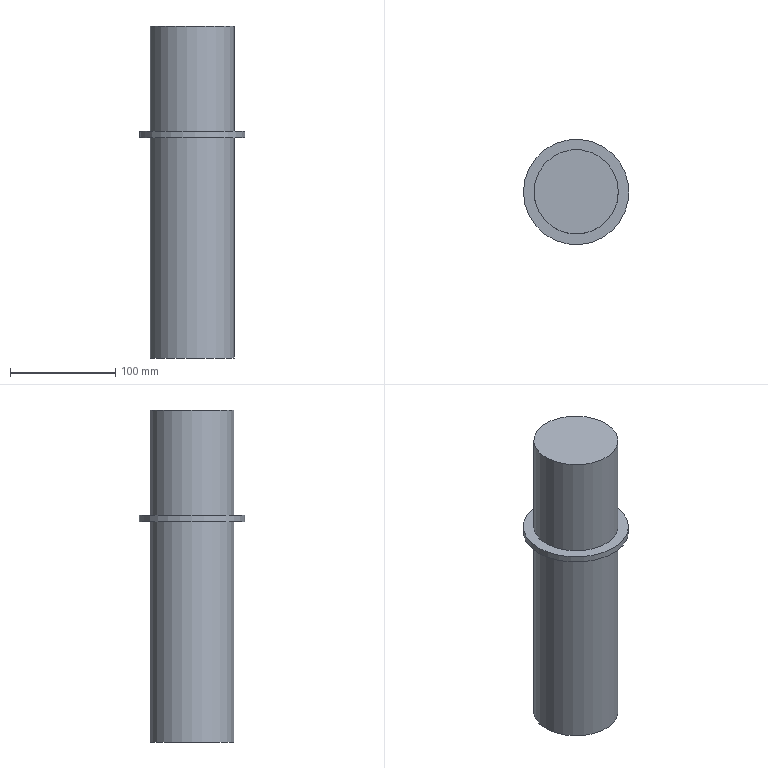Part | NX | features MAIN_BODY 2 | 1 solid | 7 faces | box 100 x 100 x 315 mm | volume 1600327 mm3 | plane 4 | cylinder 3 | commonest cylinder face diameters 80 x2 100 x1
STEP:
#1=CARTESIAN_POINT('',(-335.,-285.,370.));
#2=VERTEX_POINT('',#1);
#3=CARTESIAN_POINT('',(-295.,-285.,370.));
#4=DIRECTION('',(0.,0.,-1.));
#5=DIRECTION('',(-1.,0.,0.));
#6=AXIS2_PLACEMENT_3D('',#3,#4,#5);
#7=CIRCLE('',#6,40.);
#8=EDGE_CURVE('',#2,#2,#7,.T.);
#9=ORIENTED_EDGE('',*,*,#8,.F.);
#10=EDGE_LOOP('',(#9));
#11=FACE_BOUND('',#10,.T.);
#12=CARTESIAN_POINT('',(-255.,-285.,470.));
#13=VERTEX_POINT('',#12);
#14=CARTESIAN_POINT('',(-295.,-285.,470.));
#15=DIRECTION('',(0.,0.,1.));
#16=DIRECTION('',(1.,0.,0.));
#17=AXIS2_PLACEMENT_3D('',#14,#15,#16);
#18=CIRCLE('',#17,40.);
#19=EDGE_CURVE('',#13,#13,#18,.F.);
#20=ORIENTED_EDGE('',*,*,#19,.T.);
#21=EDGE_LOOP('',(#20));
#22=FACE_BOUND('',#21,.T.);
#23=CARTESIAN_POINT('',(-295.,-285.,463.));
#24=DIRECTION('',(0.,0.,-1.));
#25=DIRECTION('',(-1.,0.,0.));
#26=AXIS2_PLACEMENT_3D('',#23,#24,#25);
#27=CYLINDRICAL_SURFACE('',#26,40.);
#28=ADVANCED_FACE('',(#11,#22),#27,.T.);
#29=ORIENTED_EDGE('',*,*,#19,.F.);
#30=EDGE_LOOP('',(#29));
#31=FACE_BOUND('',#30,.T.);
#32=CARTESIAN_POINT('',(-295.,-285.,470.));
#33=DIRECTION('',(0.,0.,1.));
#34=DIRECTION('',(1.,0.,0.));
#35=AXIS2_PLACEMENT_3D('',#32,#33,#34);
#36=PLANE('',#35);
#37=ADVANCED_FACE('',(#31),#36,.T.);
#38=CARTESIAN_POINT('',(-345.,-285.,364.));
#39=VERTEX_POINT('',#38);
#40=CARTESIAN_POINT('',(-295.,-285.,364.));
#41=DIRECTION('',(0.,0.,-1.));
#42=DIRECTION('',(-1.,0.,0.));
#43=AXIS2_PLACEMENT_3D('',#40,#41,#42);
#44=CIRCLE('',#43,50.);
#45=EDGE_CURVE('',#39,#39,#44,.F.);
#46=ORIENTED_EDGE('',*,*,#45,.T.);
#47=EDGE_LOOP('',(#46));
#48=FACE_BOUND('',#47,.T.);
#49=CARTESIAN_POINT('',(-345.,-285.,370.));
#50=VERTEX_POINT('',#49);
#51=CARTESIAN_POINT('',(-295.,-285.,370.));
#52=DIRECTION('',(0.,0.,-1.));
#53=DIRECTION('',(-1.,0.,0.));
#54=AXIS2_PLACEMENT_3D('',#51,#52,#53);
#55=CIRCLE('',#54,50.);
#56=EDGE_CURVE('',#50,#50,#55,.F.);
#57=ORIENTED_EDGE('',*,*,#56,.F.);
#58=EDGE_LOOP('',(#57));
#59=FACE_BOUND('',#58,.T.);
#60=CARTESIAN_POINT('',(-295.,-285.,364.));
#61=DIRECTION('',(0.,0.,1.));
#62=DIRECTION('',(1.,0.,0.));
#63=AXIS2_PLACEMENT_3D('',#60,#61,#62);
#64=CYLINDRICAL_SURFACE('',#63,50.);
#65=ADVANCED_FACE('',(#48,#59),#64,.T.);
#66=CARTESIAN_POINT('',(-335.,-285.,364.));
#67=VERTEX_POINT('',#66);
#68=CARTESIAN_POINT('',(-295.,-285.,364.));
#69=DIRECTION('',(0.,0.,-1.));
#70=DIRECTION('',(-1.,0.,0.));
#71=AXIS2_PLACEMENT_3D('',#68,#69,#70);
#72=CIRCLE('',#71,40.);
#73=EDGE_CURVE('',#67,#67,#72,.T.);
#74=ORIENTED_EDGE('',*,*,#73,.F.);
#75=EDGE_LOOP('',(#74));
#76=FACE_BOUND('',#75,.T.);
#77=ORIENTED_EDGE('',*,*,#45,.F.);
#78=EDGE_LOOP('',(#77));
#79=FACE_BOUND('',#78,.T.);
#80=CARTESIAN_POINT('',(-295.,-285.,364.));
#81=DIRECTION('',(0.,0.,1.));
#82=DIRECTION('',(1.,0.,0.));
#83=AXIS2_PLACEMENT_3D('',#80,#81,#82);
#84=PLANE('',#83);
#85=ADVANCED_FACE('',(#76,#79),#84,.F.);
#86=ORIENTED_EDGE('',*,*,#8,.T.);
#87=EDGE_LOOP('',(#86));
#88=FACE_BOUND('',#87,.T.);
#89=ORIENTED_EDGE('',*,*,#56,.T.);
#90=EDGE_LOOP('',(#89));
#91=FACE_BOUND('',#90,.T.);
#92=CARTESIAN_POINT('',(-295.,-285.,370.));
#93=DIRECTION('',(0.,0.,1.));
#94=DIRECTION('',(1.,0.,0.));
#95=AXIS2_PLACEMENT_3D('',#92,#93,#94);
#96=PLANE('',#95);
#97=ADVANCED_FACE('',(#88,#91),#96,.T.);
#98=CARTESIAN_POINT('',(-335.,-285.,155.));
#99=VERTEX_POINT('',#98);
#100=CARTESIAN_POINT('',(-295.,-285.,155.));
#101=DIRECTION('',(0.,0.,-1.));
#102=DIRECTION('',(-1.,0.,0.));
#103=AXIS2_PLACEMENT_3D('',#100,#101,#102);
#104=CIRCLE('',#103,40.);
#105=EDGE_CURVE('',#99,#99,#104,.F.);
#106=ORIENTED_EDGE('',*,*,#105,.F.);
#107=EDGE_LOOP('',(#106));
#108=FACE_BOUND('',#107,.T.);
#109=CARTESIAN_POINT('',(-295.,-285.,155.));
#110=DIRECTION('',(0.,0.,1.));
#111=DIRECTION('',(1.,0.,0.));
#112=AXIS2_PLACEMENT_3D('',#109,#110,#111);
#113=PLANE('',#112);
#114=ADVANCED_FACE('',(#108),#113,.F.);
#115=ORIENTED_EDGE('',*,*,#73,.T.);
#116=EDGE_LOOP('',(#115));
#117=FACE_BOUND('',#116,.T.);
#118=ORIENTED_EDGE('',*,*,#105,.T.);
#119=EDGE_LOOP('',(#118));
#120=FACE_BOUND('',#119,.T.);
#121=CARTESIAN_POINT('',(-295.,-285.,219.));
#122=DIRECTION('',(0.,0.,1.));
#123=DIRECTION('',(1.,0.,0.));
#124=AXIS2_PLACEMENT_3D('',#121,#122,#123);
#125=CYLINDRICAL_SURFACE('',#124,40.);
#126=ADVANCED_FACE('',(#117,#120),#125,.T.);
#127=CLOSED_SHELL('',(#28,#37,#65,#85,#97,#114,#126));
#128=MANIFOLD_SOLID_BREP('',#127);
#129=(LENGTH_UNIT()NAMED_UNIT(*)SI_UNIT(.MILLI.,.METRE.));
#130=UNCERTAINTY_MEASURE_WITH_UNIT(LENGTH_MEASURE(0.00001),#129,'','');
#131=(NAMED_UNIT(*)PLANE_ANGLE_UNIT()SI_UNIT($,.RADIAN.));
#132=(NAMED_UNIT(*)SI_UNIT($,.STERADIAN.)SOLID_ANGLE_UNIT());
#133=(GEOMETRIC_REPRESENTATION_CONTEXT(3)GLOBAL_UNCERTAINTY_ASSIGNED_CONTEXT((#130))GLOBAL_UNIT_ASSIGNED_CONTEXT((#129,#131,#132))REPRESENTATION_CONTEXT('',''));
#134=ADVANCED_BREP_SHAPE_REPRESENTATION('',(#128),#133);